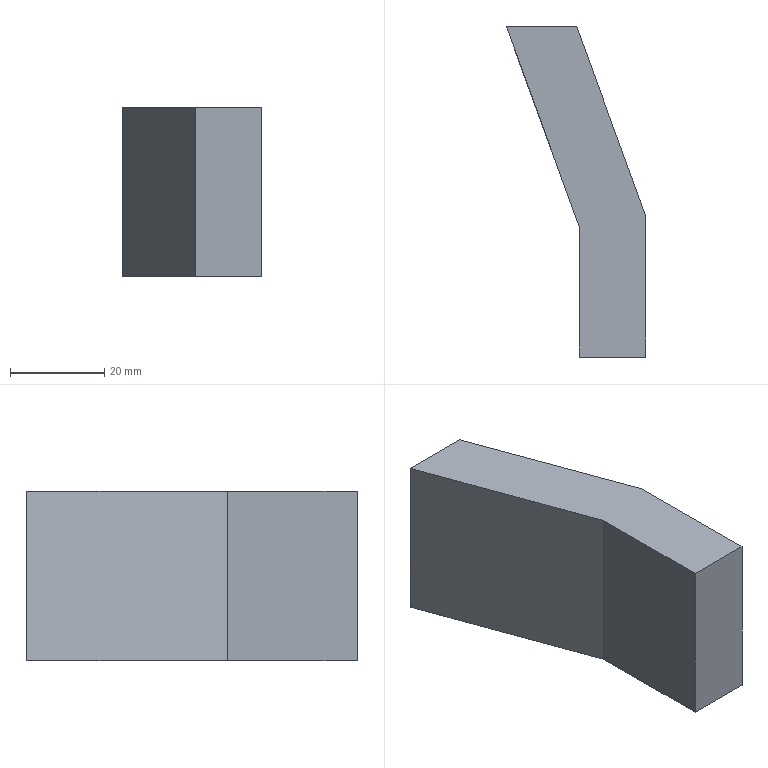Part | NX | features solid 2 | 1 solid | 8 faces | box 29.466 x 70 x 36 mm | volume 36615 mm3 | plane 8
STEP:
#1=CARTESIAN_POINT('',(344.534,0.,9.));
#2=VERTEX_POINT('',#1);
#3=CARTESIAN_POINT('',(359.432,0.,9.));
#4=VERTEX_POINT('',#3);
#5=CARTESIAN_POINT('',(344.534,0.,9.));
#6=DIRECTION('',(1.,0.,0.));
#7=VECTOR('',#6,1000.);
#8=LINE('',#5,#7);
#9=EDGE_CURVE('',#2,#4,#8,.T.);
#10=ORIENTED_EDGE('',*,*,#9,.F.);
#11=CARTESIAN_POINT('',(344.534,0.,45.));
#12=VERTEX_POINT('',#11);
#13=CARTESIAN_POINT('',(344.534,0.,45.));
#14=DIRECTION('',(0.,0.,-1.));
#15=VECTOR('',#14,1000.);
#16=LINE('',#13,#15);
#17=EDGE_CURVE('',#12,#2,#16,.T.);
#18=ORIENTED_EDGE('',*,*,#17,.F.);
#19=CARTESIAN_POINT('',(359.432,0.,45.));
#20=VERTEX_POINT('',#19);
#21=CARTESIAN_POINT('',(344.534,0.,45.));
#22=DIRECTION('',(1.,0.,0.));
#23=VECTOR('',#22,1000.);
#24=LINE('',#21,#23);
#25=EDGE_CURVE('',#12,#20,#24,.T.);
#26=ORIENTED_EDGE('',*,*,#25,.T.);
#27=CARTESIAN_POINT('',(359.432,0.,45.));
#28=DIRECTION('',(0.,0.,-1.));
#29=VECTOR('',#28,1000.);
#30=LINE('',#27,#29);
#31=EDGE_CURVE('',#20,#4,#30,.T.);
#32=ORIENTED_EDGE('',*,*,#31,.T.);
#33=EDGE_LOOP('',(#10,#18,#26,#32));
#34=FACE_BOUND('',#33,.T.);
#35=CARTESIAN_POINT('',(344.534,0.,45.));
#36=DIRECTION('',(0.,1.,0.));
#37=DIRECTION('',(0.,0.,1.));
#38=AXIS2_PLACEMENT_3D('',#35,#36,#37);
#39=PLANE('',#38);
#40=ADVANCED_FACE('',(#34),#39,.T.);
#41=CARTESIAN_POINT('',(360.,-42.494,9.));
#42=VERTEX_POINT('',#41);
#43=CARTESIAN_POINT('',(344.534,0.,9.));
#44=DIRECTION('',(0.342,-0.9397,0.));
#45=VECTOR('',#44,1000.);
#46=LINE('',#43,#45);
#47=EDGE_CURVE('',#2,#42,#46,.T.);
#48=ORIENTED_EDGE('',*,*,#47,.T.);
#49=CARTESIAN_POINT('',(360.,-42.494,45.));
#50=VERTEX_POINT('',#49);
#51=CARTESIAN_POINT('',(360.,-42.494,45.));
#52=DIRECTION('',(0.,0.,-1.));
#53=VECTOR('',#52,1000.);
#54=LINE('',#51,#53);
#55=EDGE_CURVE('',#50,#42,#54,.T.);
#56=ORIENTED_EDGE('',*,*,#55,.F.);
#57=CARTESIAN_POINT('',(344.534,0.,45.));
#58=DIRECTION('',(0.342,-0.9397,0.));
#59=VECTOR('',#58,1000.);
#60=LINE('',#57,#59);
#61=EDGE_CURVE('',#12,#50,#60,.T.);
#62=ORIENTED_EDGE('',*,*,#61,.F.);
#63=ORIENTED_EDGE('',*,*,#17,.T.);
#64=EDGE_LOOP('',(#48,#56,#62,#63));
#65=FACE_BOUND('',#64,.T.);
#66=CARTESIAN_POINT('',(344.534,0.,45.));
#67=DIRECTION('',(0.9397,0.342,0.));
#68=DIRECTION('',(-0.342,0.9397,0.));
#69=AXIS2_PLACEMENT_3D('',#66,#67,#68);
#70=PLANE('',#69);
#71=ADVANCED_FACE('',(#65),#70,.F.);
#72=CARTESIAN_POINT('',(360.,-70.,9.));
#73=VERTEX_POINT('',#72);
#74=CARTESIAN_POINT('',(360.,-42.494,9.));
#75=DIRECTION('',(0.,-1.,0.));
#76=VECTOR('',#75,1000.);
#77=LINE('',#74,#76);
#78=EDGE_CURVE('',#42,#73,#77,.T.);
#79=ORIENTED_EDGE('',*,*,#78,.T.);
#80=CARTESIAN_POINT('',(360.,-70.,45.));
#81=VERTEX_POINT('',#80);
#82=CARTESIAN_POINT('',(360.,-70.,45.));
#83=DIRECTION('',(0.,0.,-1.));
#84=VECTOR('',#83,1000.);
#85=LINE('',#82,#84);
#86=EDGE_CURVE('',#81,#73,#85,.T.);
#87=ORIENTED_EDGE('',*,*,#86,.F.);
#88=CARTESIAN_POINT('',(360.,-42.494,45.));
#89=DIRECTION('',(0.,-1.,0.));
#90=VECTOR('',#89,1000.);
#91=LINE('',#88,#90);
#92=EDGE_CURVE('',#50,#81,#91,.T.);
#93=ORIENTED_EDGE('',*,*,#92,.F.);
#94=ORIENTED_EDGE('',*,*,#55,.T.);
#95=EDGE_LOOP('',(#79,#87,#93,#94));
#96=FACE_BOUND('',#95,.T.);
#97=CARTESIAN_POINT('',(360.,-42.494,45.));
#98=DIRECTION('',(1.,0.,0.));
#99=DIRECTION('',(0.,0.,-1.));
#100=AXIS2_PLACEMENT_3D('',#97,#98,#99);
#101=PLANE('',#100);
#102=ADVANCED_FACE('',(#96),#101,.F.);
#103=CARTESIAN_POINT('',(374.,-70.,9.));
#104=VERTEX_POINT('',#103);
#105=CARTESIAN_POINT('',(360.,-70.,9.));
#106=DIRECTION('',(1.,0.,0.));
#107=VECTOR('',#106,1000.);
#108=LINE('',#105,#107);
#109=EDGE_CURVE('',#73,#104,#108,.T.);
#110=ORIENTED_EDGE('',*,*,#109,.T.);
#111=CARTESIAN_POINT('',(374.,-70.,45.));
#112=VERTEX_POINT('',#111);
#113=CARTESIAN_POINT('',(374.,-70.,45.));
#114=DIRECTION('',(0.,0.,-1.));
#115=VECTOR('',#114,1000.);
#116=LINE('',#113,#115);
#117=EDGE_CURVE('',#112,#104,#116,.T.);
#118=ORIENTED_EDGE('',*,*,#117,.F.);
#119=CARTESIAN_POINT('',(360.,-70.,45.));
#120=DIRECTION('',(1.,0.,0.));
#121=VECTOR('',#120,1000.);
#122=LINE('',#119,#121);
#123=EDGE_CURVE('',#81,#112,#122,.T.);
#124=ORIENTED_EDGE('',*,*,#123,.F.);
#125=ORIENTED_EDGE('',*,*,#86,.T.);
#126=EDGE_LOOP('',(#110,#118,#124,#125));
#127=FACE_BOUND('',#126,.T.);
#128=CARTESIAN_POINT('',(360.,-70.,45.));
#129=DIRECTION('',(0.,1.,0.));
#130=DIRECTION('',(0.,0.,1.));
#131=AXIS2_PLACEMENT_3D('',#128,#129,#130);
#132=PLANE('',#131);
#133=ADVANCED_FACE('',(#127),#132,.F.);
#134=CARTESIAN_POINT('',(374.,-40.025,9.));
#135=VERTEX_POINT('',#134);
#136=CARTESIAN_POINT('',(374.,-40.025,9.));
#137=DIRECTION('',(0.,-1.,0.));
#138=VECTOR('',#137,1000.);
#139=LINE('',#136,#138);
#140=EDGE_CURVE('',#135,#104,#139,.T.);
#141=ORIENTED_EDGE('',*,*,#140,.F.);
#142=CARTESIAN_POINT('',(374.,-40.025,45.));
#143=VERTEX_POINT('',#142);
#144=CARTESIAN_POINT('',(374.,-40.025,45.));
#145=DIRECTION('',(0.,0.,-1.));
#146=VECTOR('',#145,1000.);
#147=LINE('',#144,#146);
#148=EDGE_CURVE('',#143,#135,#147,.T.);
#149=ORIENTED_EDGE('',*,*,#148,.F.);
#150=CARTESIAN_POINT('',(374.,-40.025,45.));
#151=DIRECTION('',(0.,-1.,0.));
#152=VECTOR('',#151,1000.);
#153=LINE('',#150,#152);
#154=EDGE_CURVE('',#143,#112,#153,.T.);
#155=ORIENTED_EDGE('',*,*,#154,.T.);
#156=ORIENTED_EDGE('',*,*,#117,.T.);
#157=EDGE_LOOP('',(#141,#149,#155,#156));
#158=FACE_BOUND('',#157,.T.);
#159=CARTESIAN_POINT('',(374.,-40.025,45.));
#160=DIRECTION('',(1.,0.,0.));
#161=DIRECTION('',(0.,0.,-1.));
#162=AXIS2_PLACEMENT_3D('',#159,#160,#161);
#163=PLANE('',#162);
#164=ADVANCED_FACE('',(#158),#163,.T.);
#165=CARTESIAN_POINT('',(330.439,79.658,9.));
#166=DIRECTION('',(0.342,-0.9397,0.));
#167=VECTOR('',#166,1000.);
#168=LINE('',#165,#167);
#169=EDGE_CURVE('',#4,#135,#168,.T.);
#170=ORIENTED_EDGE('',*,*,#169,.F.);
#171=ORIENTED_EDGE('',*,*,#31,.F.);
#172=CARTESIAN_POINT('',(330.439,79.658,45.));
#173=DIRECTION('',(0.342,-0.9397,0.));
#174=VECTOR('',#173,1000.);
#175=LINE('',#172,#174);
#176=EDGE_CURVE('',#20,#143,#175,.T.);
#177=ORIENTED_EDGE('',*,*,#176,.T.);
#178=ORIENTED_EDGE('',*,*,#148,.T.);
#179=EDGE_LOOP('',(#170,#171,#177,#178));
#180=FACE_BOUND('',#179,.T.);
#181=CARTESIAN_POINT('',(330.439,79.658,45.));
#182=DIRECTION('',(0.9397,0.342,0.));
#183=DIRECTION('',(-0.342,0.9397,0.));
#184=AXIS2_PLACEMENT_3D('',#181,#182,#183);
#185=PLANE('',#184);
#186=ADVANCED_FACE('',(#180),#185,.T.);
#187=ORIENTED_EDGE('',*,*,#25,.F.);
#188=ORIENTED_EDGE('',*,*,#61,.T.);
#189=ORIENTED_EDGE('',*,*,#92,.T.);
#190=ORIENTED_EDGE('',*,*,#123,.T.);
#191=ORIENTED_EDGE('',*,*,#154,.F.);
#192=ORIENTED_EDGE('',*,*,#176,.F.);
#193=EDGE_LOOP('',(#187,#188,#189,#190,#191,#192));
#194=FACE_BOUND('',#193,.T.);
#195=CARTESIAN_POINT('',(353.295,-10.458,45.));
#196=DIRECTION('',(0.,0.,1.));
#197=DIRECTION('',(1.,0.,0.));
#198=AXIS2_PLACEMENT_3D('',#195,#196,#197);
#199=PLANE('',#198);
#200=ADVANCED_FACE('',(#194),#199,.T.);
#201=ORIENTED_EDGE('',*,*,#9,.T.);
#202=ORIENTED_EDGE('',*,*,#169,.T.);
#203=ORIENTED_EDGE('',*,*,#140,.T.);
#204=ORIENTED_EDGE('',*,*,#109,.F.);
#205=ORIENTED_EDGE('',*,*,#78,.F.);
#206=ORIENTED_EDGE('',*,*,#47,.F.);
#207=EDGE_LOOP('',(#201,#202,#203,#204,#205,#206));
#208=FACE_BOUND('',#207,.T.);
#209=CARTESIAN_POINT('',(353.295,-10.458,9.));
#210=DIRECTION('',(0.,0.,1.));
#211=DIRECTION('',(1.,0.,0.));
#212=AXIS2_PLACEMENT_3D('',#209,#210,#211);
#213=PLANE('',#212);
#214=ADVANCED_FACE('',(#208),#213,.F.);
#215=CLOSED_SHELL('',(#40,#71,#102,#133,#164,#186,#200,#214));
#216=MANIFOLD_SOLID_BREP('',#215);
#217=(LENGTH_UNIT()NAMED_UNIT(*)SI_UNIT(.MILLI.,.METRE.));
#218=UNCERTAINTY_MEASURE_WITH_UNIT(LENGTH_MEASURE(0.00001),#217,'','');
#219=(NAMED_UNIT(*)PLANE_ANGLE_UNIT()SI_UNIT($,.RADIAN.));
#220=(NAMED_UNIT(*)SI_UNIT($,.STERADIAN.)SOLID_ANGLE_UNIT());
#221=(GEOMETRIC_REPRESENTATION_CONTEXT(3)GLOBAL_UNCERTAINTY_ASSIGNED_CONTEXT((#218))GLOBAL_UNIT_ASSIGNED_CONTEXT((#217,#219,#220))REPRESENTATION_CONTEXT('',''));
#222=ADVANCED_BREP_SHAPE_REPRESENTATION('',(#216),#221);